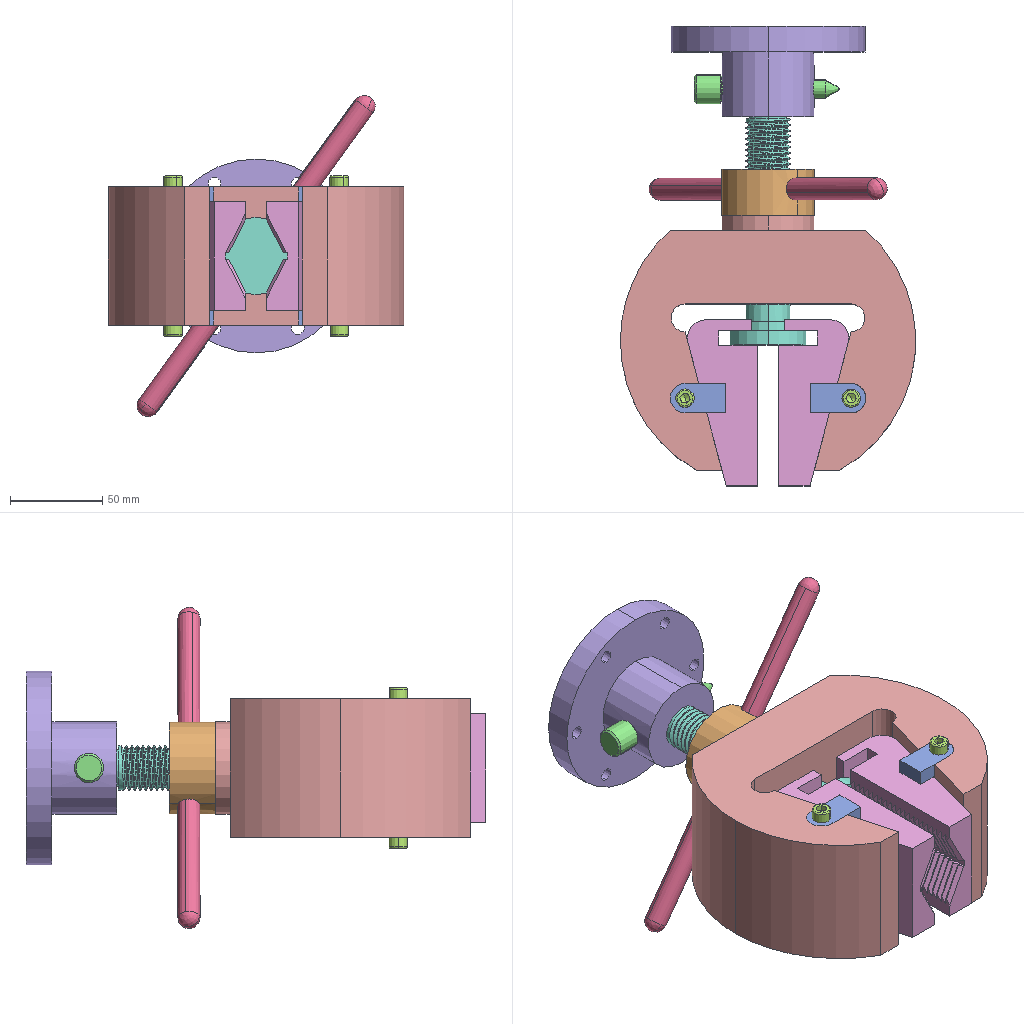Assembly | SolidWorks | 9 different items | 14 placed | box 160 x 249 x 174 mm
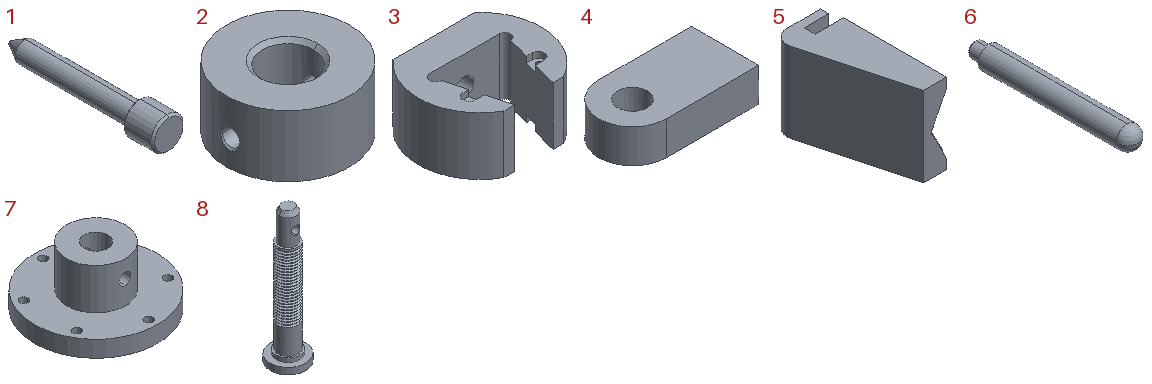Parts list (item | name | quantity | size | volume | features):
1 | - | x1 | 16 x 78.492 x 16 mm | 7592 mm3 | features Chamfer 1, Revolution 1
2 | - | x1 | 50 x 50 x 25 mm | 39286 mm3 | features 3DProfileFeature 2, HoleWzd 2, Extrusion 1
3 | - | x1 | 160 x 138 x 75 mm | 835946 mm3 | features ICE 6, 3DProfileFeature 1, Extrusion 1, HoleWzd 1
4 | - | x4 | 30 x 16 x 8 mm | 3312 mm3 | features Extrusion 1
5 | - | x2 | 37.984 x 90 x 59 mm | 121920 mm3 | features ICE 5, Extrusion 1
6 | - | x2 | 12 x 89 x 12 mm | 9325 mm3 | features Chamfer 1, Revolution 1
7 | - | x1 | 105 x 105 x 49 mm | 173332 mm3 | features ICE 2, Extrusion 1
8 | - | x1 | 42 x 42 x 158.7 mm | 67679 mm3 | features ICE 4, Chamfer 1, Extrusion 1, SweepThread 1
9 | hexagon socket head cap screws gb | x1 | - | - | -
Mates (type | each side: item.copy, entity, surface, feature):
Concentric | 4.1 face cylinder Boss-Extrude1 | 3.1 face cylinder M6 Tapped Hole1
Coincident | 3.1 face plane Cut-Extrude4 | 4.1 face plane Boss-Extrude1 | 2 times
Concentric | 3.1 face cylinder M6 Tapped Hole1 | 4.2 face cylinder Boss-Extrude1
Coincident | 3.1 face plane Cut-Extrude4 | 4.2 face plane Boss-Extrude1 | 2 times
Concentric | 3.1 face cylinder M6 Tapped Hole1 | 4.3 face cylinder Boss-Extrude1
Coincident | 3.1 face plane Cut-Extrude3 | 4.3 face plane Boss-Extrude1 | 2 times
Concentric | 3.1 face cylinder M6 Tapped Hole1 | 4.4 face cylinder Boss-Extrude1
Coincident | 3.1 face plane Cut-Extrude3 | 4.4 face plane Boss-Extrude1 | 2 times
Coincident | 3.1 face plane Cut-Extrude2 | 5.1 face plane Boss-Extrude1
Coincident | 4.3 face plane Boss-Extrude1 | 5.1 face plane Boss-Extrude1
Coincident | 3.1 face plane Cut-Extrude2 | 5.2 face plane Boss-Extrude1
Coincident | 5.1 face plane Boss-Extrude1 | 5.2 face plane Boss-Extrude1 | 2 times
Coincident | 5.2 face plane Boss-Extrude1 | 8.1 face plane Boss-Extrude1
Concentric | 3.1 face cylinder Cut-Extrude5 | 8.1 face cylinder Boss-Extrude3
Concentric | 3.1 face cylinder Boss-Extrude4 | 2.1 face cylinder Boss-Extrude1
Coincident | 3.1 face plane Boss-Extrude4 | 2.1 face plane Boss-Extrude1
Concentric | 2.1 face cylinder Boss-Extrude1 | 7.1 face cylinder Boss-Extrude2
Concentric | 8.1 face cylinder Cut-Extrude1 | 7.1 face cylinder Cut-Extrude1
Concentric | 7.1 face cylinder Cut-Extrude1 | 1.1 face cylinder Revolve1
Tangent | 7.1 face cylinder Boss-Extrude2 | 1.1 face plane Revolve1
Concentric | 2.1 face cylinder M8 Tapped Hole1 | 6.1 face cylinder Revolve1
Tangent | 2.1 face cylinder Boss-Extrude1 | 6.1 face plane Revolve1
Concentric | 2.1 face cylinder M8 Tapped Hole1 | 6.2 face cylinder Revolve1
Tangent | 2.1 face cylinder Boss-Extrude1 | 6.2 face plane Revolve1
Screw | 8.1 face cylinder Boss-Extrude3 | 2.1 face cylinder Boss-Extrude1
Parallel | 7.1 plane | 5.1 face plane Boss-Extrude1